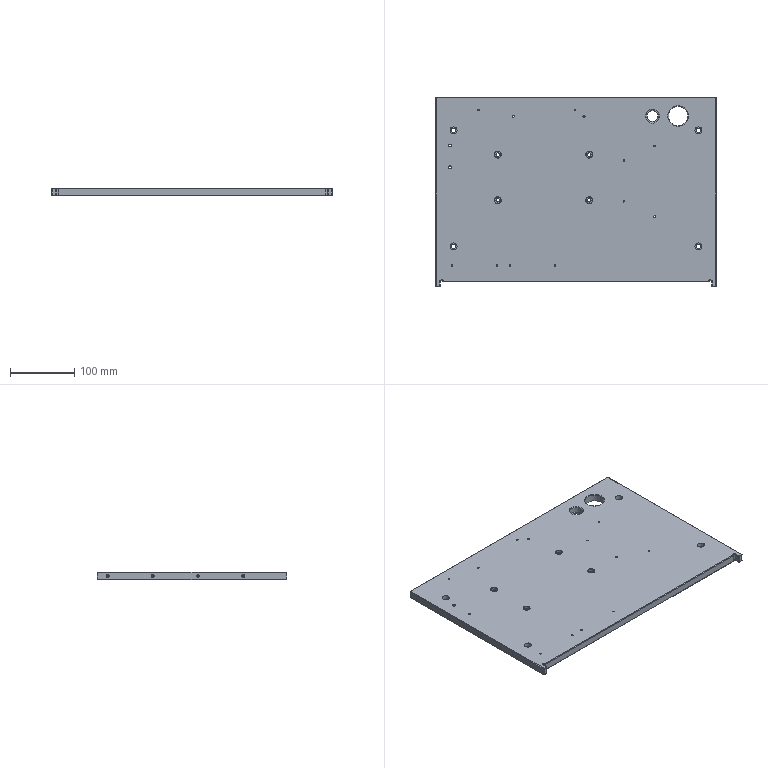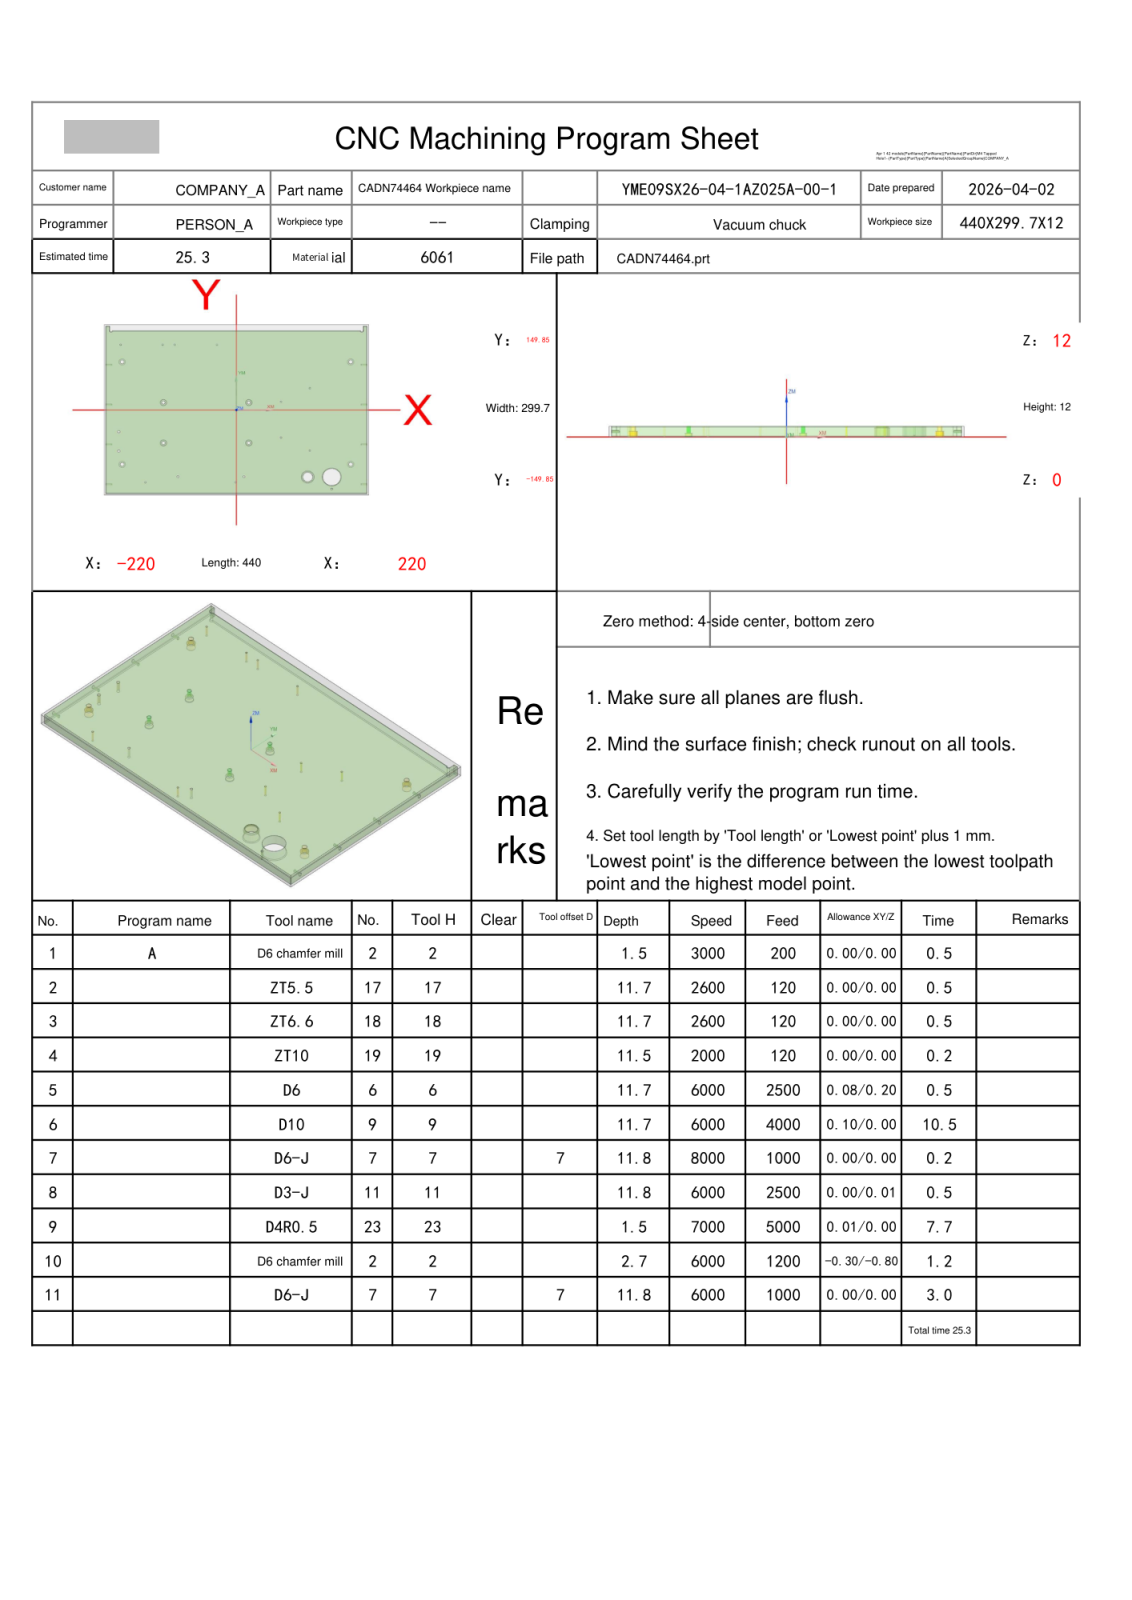NC program | NX | posted by the shop | part box 435 x 294.7 x 12 mm
Lines 3076 to 4772 of 24066:
N9 T23 M06
(D4R0.5  D=4. R=0.5 H=23 ce=0.01 di=0.00)
G00 G90 G54 X218.164 Y-120.194 M03 S7000
G43 H23 Z32.
M08
Z13.5
G01 Y-146.479 Z12.122 F5000.
X218.104 Y-146.811 Z12.105
X217.979 Y-147.124 Z12.087
X217.793 Y-147.405 Z12.069
X217.555 Y-147.643 Z12.052
X217.274 Y-147.829 Z12.034
X216.961 Y-147.954 Z12.016
X216.629 Y-148.014 Z11.999
X216.5 Z11.992
X-216.5
G02 X-218.164 Y-146.35 I0.0 J1.664
G01 Y146.35
G02 X-216.5 Y148.014 I1.664 J0.0
G01 X-211.5
G02 X-209.836 Y146.35 I0.0 J-1.664
G01 Y139.35
G03 X-208.5 Y138.014 I1.336 J0.0
X-207.23 Y138.937 I0.0 J1.336
G02 X-205.744 Y140.014 I1.486 J-.486
G01 X-205.742
X205.742
X205.744
G02 X207.23 Y138.937 I0.0 J-1.563
G03 X208.5 Y138.014 I1.27 J.413
X209.836 Y139.35 I0.0 J1.336
G01 Y146.35
G02 X211.5 Y148.014 I1.664 J0.0
G01 X216.5
G02 X218.164 Y146.35 I0.0 J-1.664
G01 Y-146.35
G02 X216.5 Y-148.014 I-1.664 J0.0
G01 X214.495
X212.491
X210.486 Y-148.015
X208.481 Y-148.014
X206.477 Y-148.015
X204.472 Y-148.014
X202.468 Y-148.015
X200.463
X198.458 Y-148.016
X196.454 Y-148.015
X194.449 Y-148.016
X192.444 Y-148.015
X190.44 Y-148.016
X188.435
X186.431
X184.426
X182.421 Y-148.017
X180.417 Y-148.016
X178.412 Y-148.017
X176.407
X174.403
X172.398
X170.394 Y-148.018
X168.389 Y-148.017
X166.384 Y-148.018
X164.38
X162.375
X160.37
X158.366 Y-148.019
X156.361 Y-148.018
X154.356 Y-148.019
X152.352
X150.347
X148.343 Z11.991
X146.338 Y-148.02
X144.333 Y-148.019
X142.329 Y-148.02
X140.324
X138.319
X136.315
X134.31 Y-148.021
X132.306 Y-148.02
X130.301 Y-148.021
X128.296
X126.292
X124.287
X122.282 Y-148.022
X120.278 Y-148.021
X118.273 Y-148.022
X116.269
X114.264
X112.259
X110.255 Y-148.023
X108.25 Y-148.022
X106.245 Y-148.023
X104.241
X102.236
X100.231
X98.227
X96.222
X94.218 Y-148.024
X92.213
X90.208
X88.204
X86.199
X84.194
X82.19 Y-148.025
X80.185
X78.181
X76.176
X74.171
X72.167
X70.162 Y-148.026
X68.157
X66.153
X64.148
X62.144
X60.139
X58.134 Y-148.027
X56.13
X54.125
X52.12
X50.116
X48.111
X46.106 Y-148.028
X44.102
X42.097
X40.093
X38.088
X36.083
X34.079
X32.074
X30.069 Y-148.029 Z11.99
X28.065
X26.06
X24.056
X22.051
X20.046
X18.042 Y-148.03
X16.037
X14.032
X12.028
X10.023
X8.019
X6.014
X4.009
X2.005 Y-148.031
X0.0
X-2.005
X-4.009
X-6.014
X-8.019
X-10.023 Y-148.032
X-12.028 Y-148.031
X-14.032 Y-148.032
X-16.037
X-18.042
X-20.046
X-22.051 Y-148.033
X-24.056 Y-148.032
X-26.06 Y-148.033
X-28.065
X-30.069
X-32.074
X-34.079
X-36.083
X-38.088 Y-148.034
X-40.093 Y-148.033
X-42.097 Y-148.034
X-44.102
X-46.106
X-48.111
X-50.116 Y-148.035
X-52.12 Y-148.034
X-54.125 Y-148.035
X-56.13 Y-148.034
X-58.134 Y-148.035
X-60.139
X-62.144
X-64.148
X-66.153 Y-148.036
X-68.157 Y-148.035
X-70.162 Y-148.036
X-72.167
X-74.171
X-76.176
X-78.181 Y-148.037
X-80.185 Y-148.036
X-82.19 Y-148.037
X-84.194 Y-148.036
X-86.199 Y-148.037
X-88.204 Z11.989
X-90.208
X-92.213
X-94.218 Y-148.038
X-96.222 Y-148.037
X-98.227 Y-148.038
X-100.231 Y-148.037
X-102.236 Y-148.038
X-104.241
X-106.245 Y-148.039
X-108.25 Y-148.038
X-110.255 Y-148.039
X-112.259 Y-148.038
X-114.264 Y-148.039
X-116.269
X-118.273
X-120.278
X-122.282 Y-148.04
X-124.287 Y-148.039
X-126.292 Y-148.04
X-128.296 Y-148.039
X-130.301 Y-148.04
X-132.306
X-134.31
X-136.315
X-138.319 Y-148.041
X-140.324 Y-148.04
X-142.329 Y-148.041
X-144.333
X-146.338
X-148.343
X-150.347 Y-148.042
X-152.352 Y-148.041
X-154.356 Y-148.042
X-156.361 Y-148.041
X-158.366 Y-148.042
X-160.37
X-162.375
X-164.38
X-166.384 Y-148.043
X-168.389 Y-148.042
X-170.394 Y-148.043
X-172.398 Y-148.042
X-174.403 Y-148.043
X-176.407
X-178.412 Y-148.044
X-180.417 Y-148.043
X-182.421 Y-148.044
X-184.426 Y-148.043
X-186.431 Y-148.044
X-188.435
X-190.44
X-192.444
X-194.449 Y-148.045
X-196.454 Y-148.044
X-198.458 Y-148.045
X-200.463 Y-148.044
X-202.468 Y-148.045
X-204.472
X-206.477 Z11.988
X-208.481
X-210.486 Y-148.046
X-212.491 Y-148.045
X-214.495 Y-148.046
X-216.5 Y-148.045
X-216.621 Y-148.042
X-216.741 Y-148.028
X-216.86 Y-148.007
X-216.978 Y-147.977
X-217.093 Y-147.939
X-217.204 Y-147.892
X-217.313 Y-147.838
X-217.417 Y-147.776
X-217.516 Y-147.708
X-217.61 Y-147.631
X-217.699 Y-147.549
X-217.781 Y-147.46
X-217.858 Y-147.366
X-217.926 Y-147.267
X-217.989 Y-147.163
X-218.042 Y-147.054
X-218.089 Y-146.943
X-218.127 Y-146.828
X-218.157 Y-146.711
X-218.178 Y-146.591
X-218.192 Y-146.471
X-218.196 Y-146.35
Y-144.345
Y-142.34
X-218.197 Y-140.336
X-218.196 Y-138.331
X-218.197 Y-136.326
X-218.196 Y-134.321
X-218.197 Y-132.316
Y-130.312
X-218.198 Y-128.307
X-218.197 Y-126.302
X-218.198 Y-124.297
X-218.197 Y-122.292
X-218.198 Y-120.288
Y-118.283
Y-116.278
Y-114.273
X-218.199 Y-112.268
X-218.198 Y-110.264
X-218.199 Y-108.259
X-218.198 Y-106.254
X-218.199 Y-104.249
Y-102.245
Y-100.24
Y-98.235
X-218.2 Y-96.23
X-218.199 Y-94.225
X-218.2 Y-92.221
X-218.199 Y-90.216
X-218.2 Y-88.211
Y-86.206
Y-84.201
Y-82.197
X-218.201 Y-80.192
X-218.2 Y-78.187
X-218.201 Y-76.182
Y-74.177
Y-72.173
Y-70.168
X-218.202 Y-68.163
X-218.201 Y-66.158
X-218.202 Y-64.153
X-218.201 Y-62.149
X-218.202 Y-60.144
Y-58.139
Y-56.134
Y-54.129
X-218.203 Y-52.125
X-218.202 Y-50.12
X-218.203 Y-48.115
X-218.202 Y-46.11
X-218.203 Y-44.105
Y-42.101 Z11.987
Y-40.096
Y-38.091
X-218.204 Y-36.086
X-218.203 Y-34.082
X-218.204 Y-32.077
Y-30.072
Y-28.067
Y-26.062
Y-24.058
Y-22.053
X-218.205 Y-20.048
X-218.204 Y-18.043
X-218.205 Y-16.038
Y-14.034
Y-12.029
Y-10.024
Y-8.019
Y-6.014
X-218.206 Y-4.01
Y-2.005
Y0.0
Y2.005
Y4.01
Y6.014
Y8.019
Y10.024
X-218.207 Y12.029
Y14.034
Y16.038
Y18.043
Y20.048
Y22.053
X-218.208 Y24.058
X-218.207 Y26.062
X-218.208 Y28.067
Y30.072
Y32.077
Y34.082
Y36.086
Y38.091
X-218.209 Y40.096
Y42.101
Y44.105
Y46.11
Y48.115
Y50.12
Y52.125
Y54.129
X-218.21 Y56.134
Y58.139
Y60.144
Y62.149
Y64.153
Y66.158
Y68.163
Y70.168
X-218.211 Y72.173
Y74.177
Y76.182 Z11.986
Y78.187
Y80.192
Y82.197
Y84.201
Y86.206
X-218.212 Y88.211
Y90.216
Y92.221
Y94.225
Y96.23
Y98.235
Y100.24
Y102.245
X-218.213 Y104.249
Y106.254
Y108.259
Y110.264
Y112.268
Y114.273
Y116.278
Y118.283
X-218.214 Y120.288
X-218.213 Y122.292
X-218.214 Y124.297
Y126.302
Y128.307
Y130.312
Y132.316
Y134.321
X-218.215 Y136.326
X-218.214 Y138.331
X-218.215 Y140.336
Y142.34
Y144.345
Y146.35
X-218.211 Y146.472
X-218.197 Y146.594
X-218.176 Y146.715
X-218.145 Y146.833
X-218.107 Y146.949
X-218.06 Y147.062
X-218.005 Y147.172
X-217.943 Y147.277
X-217.873 Y147.378
X-217.796 Y147.473
X-217.713 Y147.563
X-217.623 Y147.646
X-217.528 Y147.723
X-217.427 Y147.793
X-217.322 Y147.855
X-217.212 Y147.91
X-217.099 Y147.957
X-216.983 Y147.996
X-216.865 Y148.026
X-216.744 Y148.048
X-216.622 Y148.061
X-216.5 Y148.065
X-215.25
X-214.
X-212.75
X-211.5
X-211.378 Y148.061
X-211.256 Y148.048
X-211.135 Y148.026
X-211.017 Y147.996
X-210.901 Y147.957
X-210.787 Y147.91
X-210.678 Y147.856
X-210.573 Y147.793
X-210.472 Y147.723
X-210.377 Y147.646
X-210.287 Y147.563
X-210.204 Y147.473
X-210.127 Y147.378
X-210.057 Y147.277
X-209.994 Y147.172
X-209.94 Y147.063
X-209.893 Y146.949
X-209.854 Y146.833
X-209.824 Y146.715
X-209.802 Y146.594
X-209.789 Y146.472
X-209.785 Y146.35
Y144.6
X-209.784 Y142.85
X-209.785 Y141.1
X-209.784 Y139.35
X-209.78 Y139.251
X-209.769 Y139.152
X-209.75 Y139.055
X-209.723 Y138.959
X-209.689 Y138.866
X-209.648 Y138.775
X-209.6 Y138.688
X-209.546 Y138.605
X-209.485 Y138.527
X-209.419 Y138.453
X-209.346 Y138.385
X-209.269 Y138.322
X-209.188 Y138.266
X-209.102 Y138.216
X-209.01 Y138.172
X-208.915 Y138.135
X-208.818 Y138.106
X-208.718 Y138.085
X-208.617 Y138.071
X-208.516 Y138.066
X-208.414 Y138.069
X-208.313 Y138.08
X-208.213 Y138.099
X-208.115 Y138.125
X-208.019 Y138.16
X-207.926 Y138.201
X-207.837 Y138.251
X-207.752 Y138.307
X-207.672 Y138.369
X-207.597 Y138.438
X-207.527 Y138.512
X-207.464 Y138.592
X-207.407 Y138.676
X-207.357 Y138.765
X-207.315 Y138.857
X-207.276 Y138.963
X-207.273 Y138.973
X-207.233 Y139.082
X-207.186 Y139.187
X-207.157 Y139.244
X-207.125 Y139.298
X-207.092 Y139.353
X-207.055 Y139.406
X-207.018 Y139.457
X-206.978 Y139.506
X-206.935 Y139.555
X-206.891 Y139.601
X-206.845 Y139.646
X-206.798 Y139.688
X-206.748 Y139.729
X-206.697 Y139.767
X-206.645 Y139.804
X-206.59 Y139.838
X-206.535 Y139.87
X-206.479 Y139.9
X-206.421 Y139.927
X-206.362 Y139.952
X-206.303 Y139.975
X-206.242 Y139.995
X-206.181 Y140.013
X-206.118 Y140.028
X-206.056 Y140.041
X-205.994 Y140.051
X-205.891 Y140.062
X-205.788 Y140.066
X-205.765 Y140.067
X-205.742 Y140.066
X-203.744 Y140.065
X-201.747 Y140.066
X-199.749
X-197.752 Y140.067
X-195.754 Y140.066
X-193.757 Y140.067
X-191.759 Y140.066
X-189.762 Y140.067
X-187.765 Y140.066
X-185.767 Y140.067
X-183.77
X-181.772 Y140.068
X-179.775 Y140.067 Z11.985
X-177.777 Y140.068
X-175.78 Y140.067
X-173.782 Y140.068
X-171.785 Y140.067
X-169.787 Y140.068
X-167.79
X-165.792 Y140.069
X-163.795 Y140.068
X-161.797 Y140.069
X-159.8 Y140.068
X-157.802 Y140.069
X-155.805 Y140.068
X-153.807 Y140.069
X-151.81
X-149.812
X-147.815
X-145.817 Y140.07
X-143.82 Y140.069
X-141.822 Y140.07
X-139.825 Y140.069
X-137.827 Y140.07
X-135.83 Y140.069
X-133.832 Y140.07
X-131.835
X-129.837 Y140.071
X-127.84 Y140.07
X-125.842 Y140.071
X-123.845 Y140.07
X-121.847 Y140.071
X-119.85 Y140.07
X-117.852 Y140.071
X-115.855
X-113.857 Y140.072
X-111.86 Y140.071
X-109.862 Y140.072
X-107.865 Y140.071
X-105.867 Y140.072
X-103.87 Y140.071
X-101.872 Y140.072
X-99.875
X-97.877
X-95.88
X-93.882 Y140.073
X-91.885 Y140.072
X-89.887 Y140.073
X-87.89 Y140.072
X-85.892 Y140.073
X-83.895
X-81.897
X-79.9
X-77.902 Y140.074
X-75.905 Y140.073
X-73.907 Y140.074
X-71.91 Y140.073
X-69.912 Y140.074
X-67.915
X-65.917
X-63.92
X-61.922 Y140.075 Z11.984
X-59.925 Y140.074
X-57.927 Y140.075
X-55.93 Y140.074
X-53.932 Y140.075
X-51.935
X-49.937
X-47.94
X-45.942
X-43.945
X-41.947 Y140.076
X-39.95 Y140.075
X-37.952 Y140.076
X-35.955
X-33.957
X-31.96
X-29.962
X-27.965
X-25.967 Y140.077
X-23.97 Y140.076
X-21.972 Y140.077
X-19.975
X-17.977
X-15.98
X-13.982
X-11.985
X-9.987 Y140.078
X-7.99 Y140.077
X-5.992 Y140.078
X-3.995
X-1.997
X0.0
X1.997
X3.995
X5.992
X7.99
X9.987 Y140.079
X11.985 Y140.078
X13.982 Y140.079
X15.98
X17.977
X19.975
X21.972
X23.97
X25.967 Y140.08
X27.965 Y140.079
X29.962 Y140.08
X31.96
X33.957
X35.955
X37.952
X39.95
X41.947 Y140.081
X43.945 Y140.08
X45.942 Y140.081
X47.94
X49.937
X51.935
X53.932
X55.93 Z11.983
X57.927
X59.925
X61.922 Y140.082
X63.92
X65.917
X67.915
X69.912
X71.91
X73.907
X75.905
X77.902 Y140.083
X79.9
X81.897
X83.895
X85.892
X87.89
X89.887
X91.885
X93.882 Y140.084
X95.88
X97.877
X99.875
X101.872
X103.87
X105.867
X107.865
X109.862
X111.86 Y140.085
X113.857
X115.855
X117.852
X119.85
X121.847
X123.845
X125.842
X127.84 Y140.086
X129.837
X131.835
X133.832
X135.83
X137.827
X139.825
X141.822
X143.82 Y140.087
X145.817
X147.815
X149.812
X151.81
X153.807
X155.805
X157.802
X159.8 Y140.088
X161.797 Y140.087
X163.795 Y140.088
X165.792
X167.79
X169.787
X171.785
X173.782 Z11.982
X175.78
X177.777
X179.775 Y140.089
X181.772
X183.77
X185.767
X187.765
X189.762
X191.759
X193.757
X195.754 Y140.09
X197.752
X199.749
X201.747
X203.744
X205.742
X205.765
X205.788 Y140.089
X205.893 Y140.086
X205.997 Y140.076
X206.061 Y140.066
X206.124 Y140.053
X206.187 Y140.038
X206.25 Y140.02
X206.312 Y140.
X206.372 Y139.977
X206.432 Y139.952
X206.491 Y139.924
X206.549 Y139.894
X206.605 Y139.862
X206.66 Y139.827
X206.714 Y139.79
X206.765 Y139.751
X206.816 Y139.709
X206.864 Y139.666
X206.911 Y139.621
X206.956 Y139.573
X206.998 Y139.524
X207.039 Y139.474
X207.078 Y139.421
X207.114 Y139.368
X207.148 Y139.312
X207.18 Y139.256
X207.209 Y139.198
X207.256 Y139.091
X207.295 Y138.98
X207.302 Y138.96
X207.335 Y138.869
X207.376 Y138.781
X207.423 Y138.697
X207.476 Y138.616
X207.536 Y138.54
X207.601 Y138.468
X207.671 Y138.401
X207.746 Y138.341
X207.826 Y138.286
X207.91 Y138.237
X208.007 Y138.191
X208.108 Y138.153
X208.212 Y138.123
X208.318 Y138.103
X208.426 Y138.092
X208.534 Y138.091
X208.642 Y138.098
X208.748 Y138.115
X208.853 Y138.141
X208.956 Y138.175
X209.054 Y138.219
X209.149 Y138.27
X209.239 Y138.33
X209.324 Y138.397
X209.403 Y138.471
X209.475 Y138.552
X209.539 Y138.638
X209.597 Y138.73
X209.646 Y138.826
X209.686 Y138.926
X209.718 Y139.029
X209.741 Y139.135
X209.755 Y139.242
X209.76 Y139.35
Y141.1
Y142.85
Y144.6
X209.759 Y146.35
X209.764 Y146.474
X209.777 Y146.598
X209.799 Y146.72
X209.83 Y146.84
X209.869 Y146.958
X209.917 Y147.073
X209.972 Y147.184
X210.036 Y147.291
X210.106 Y147.393
X210.184 Y147.49
X210.269 Y147.581
X210.36 Y147.666
X210.457 Y147.744
X210.559 Y147.814
X210.666 Y147.878
X210.777 Y147.934
X210.892 Y147.981
X211.01 Y148.02
X211.13 Y148.051
X211.252 Y148.073
X211.376 Y148.086
X211.5 Y148.091
X212.75
X214.
X215.25
X216.5
X216.624 Y148.087
X216.748 Y148.073
X216.87 Y148.051
X216.991 Y148.021
X217.108 Y147.981
X217.223 Y147.934
X217.334 Y147.878
X217.441 Y147.815
X217.543 Y147.744
X217.64 Y147.666
X217.731 Y147.581
X217.816 Y147.49
X217.894 Y147.393
X217.965 Y147.291
X218.028 Y147.184
X218.084 Y147.073
X218.131 Y146.958
X218.171 Y146.841
X218.201 Y146.72
X218.224 Y146.598
X218.237 Y146.474
X218.241 Y146.35
X218.242 Y144.345
Y142.34
Y140.336
Y138.331
Y136.326
Y134.321
Y132.316
Y130.312
Y128.307
Y126.302
X218.243 Y124.297
Y122.292
Y120.288
Y118.283
Y116.278
Y114.273
Y112.268
Y110.264
X218.244 Y108.259
Y106.254
Y104.249
Y102.245
Y100.24
Y98.235
Y96.23
Y94.225
Y92.221
Y90.216
X218.245 Y88.211
Y86.206
Y84.201
Y82.197 Z11.981
Y80.192
Y78.187
Y76.182
Y74.177
Y72.173
Y70.168
X218.246 Y68.163
Y66.158
Y64.153
Y62.149
Y60.144
Y58.139
Y56.134
Y54.129
X218.247 Y52.125
X218.246 Y50.12
X218.247 Y48.115
Y46.11
Y44.105
Y42.101
Y40.096
Y38.091
Y36.086
Y34.082
X218.248 Y32.077
X218.247 Y30.072
X218.248 Y28.067
Y26.062
Y24.058
Y22.053
Y20.048
Y18.043
Y16.038
Y14.034
X218.249 Y12.029
X218.248 Y10.024
X218.249 Y8.019
Y6.014
Y4.01
Y2.005
Y0.0
Y-2.005
Y-4.01
Y-6.014
X218.25 Y-8.019
X218.249 Y-10.024
X218.25 Y-12.029
Y-14.034
Y-16.038
Y-18.043
Y-20.048
Y-22.053
X218.251 Y-24.058
X218.25 Y-26.062
X218.251 Y-28.067
X218.25 Y-30.072
X218.251 Y-32.077
Y-34.082
Y-36.086 Z11.98
Y-38.091
Y-40.096
Y-42.101
X218.252 Y-44.105
X218.251 Y-46.11
X218.252 Y-48.115
X218.251 Y-50.12
X218.252 Y-52.125
Y-54.129
Y-56.134
Y-58.139
Y-60.144
Y-62.149
X218.253 Y-64.153
X218.252 Y-66.158
X218.253 Y-68.163
X218.252 Y-70.168
X218.253 Y-72.173
Y-74.177
Y-76.182
Y-78.187
Y-80.192
Y-82.197
X218.254 Y-84.201
X218.253 Y-86.206
X218.254 Y-88.211
X218.253 Y-90.216
X218.254 Y-92.221
Y-94.225
Y-96.23
Y-98.235
Y-100.24
Y-102.245
X218.255 Y-104.249
X218.254 Y-106.254
X218.255 Y-108.259
X218.254 Y-110.264
X218.255 Y-112.268
Y-114.273
Y-116.278
Y-118.283
Y-120.288
Y-122.292
X218.256 Y-124.297
X218.255 Y-126.302
X218.256 Y-128.307
X218.255 Y-130.312
X218.256 Y-132.316
Y-134.321
Y-136.326
Y-138.331
Y-140.336
Y-142.34
X218.257 Y-144.345
X218.256 Y-146.35
X218.252 Y-146.475
X218.238 Y-146.6
X218.216 Y-146.723
X218.185 Y-146.845
X218.146 Y-146.964
X218.098 Y-147.08
X218.042 Y-147.192
X217.978 Y-147.3
X217.906 Y-147.403
X217.827 Y-147.5
X217.742 Y-147.592
X217.65 Y-147.677
X217.553 Y-147.756
X217.45 Y-147.828
X217.342 Y-147.892
X217.23 Y-147.948
X217.114 Y-147.996
X216.995 Y-148.035
X216.873 Y-148.067
X216.75 Y-148.089
X216.625 Y-148.102
X216.5 Y-148.107
X214.495
X212.491 Z11.979
X210.486
X208.481
X206.477 Y-148.108
X204.472 Y-148.107
X202.468 Y-148.108
X200.463
X198.458
X196.454
X194.449
X192.444
X190.44 Y-148.109
X188.435 Y-148.108
X186.431 Y-148.109
X184.426
X182.421
X180.417
X178.412 Y-148.11
X176.407 Y-148.109
X174.403 Y-148.11
X172.398
X170.394
X168.389
X166.384
X164.38
X162.375 Y-148.111
X160.37 Y-148.11
X158.366 Y-148.111
X156.361
X154.356
X152.352
X150.347 Y-148.112
X148.343 Y-148.111
X146.338 Y-148.112
X144.333
X142.329
X140.324
X138.319
X136.315
X134.31 Y-148.113
X132.306
X130.301
X128.296 Z11.978
X126.292
X124.287
X122.282 Y-148.114
X120.278 Y-148.113
X118.273 Y-148.114
X116.269
X114.264
X112.259
X110.255
X108.25
X106.245 Y-148.115
X104.241
X102.236
X100.231
X98.227
X96.222
X94.218
X92.213
X90.208 Y-148.116
X88.204
X86.199
X84.194
X82.19
X80.185
X78.181 Y-148.117
X76.176
X74.171
X72.167
X70.162
X68.157
X66.153
X64.148
X62.144 Y-148.118
X60.139
X58.134
X56.13
X54.125
X52.12
X50.116
X48.111 Y-148.119
X46.106
X44.102 Z11.977
X42.097
X40.093
X38.088
X36.083
X34.079 Y-148.12
X32.074
X30.069
X28.065
X26.06
X24.056
X22.051
X20.046
X18.042 Y-148.121
X16.037
X14.032
X12.028
X10.023
X8.019
X6.014
X4.009
X2.005 Y-148.122
X0.0
X-2.005
X-4.009
X-6.014
X-8.019
X-10.023
X-12.028
X-14.032 Y-148.123
X-16.037
X-18.042
X-20.046
X-22.051
X-24.056
X-26.06 Y-148.124
X-28.065 Y-148.123
X-30.069 Y-148.124
X-32.074
X-34.079
X-36.083
X-38.088
X-40.093
X-42.097 Y-148.125 Z11.976
X-44.102 Y-148.124
X-46.106 Y-148.125
X-48.111
X-50.116
X-52.12
X-54.125
X-56.13
X-58.134 Y-148.126
X-60.139 Y-148.125
X-62.144 Y-148.126
X-64.148
X-66.153
X-68.157
X-70.162
X-72.167
X-74.171 Y-148.127
X-76.176 Y-148.126
X-78.181 Y-148.127
X-80.185
X-82.19
X-84.194
X-86.199
X-88.204
X-90.208 Y-148.128
X-92.213 Y-148.127
X-94.218 Y-148.128
X-96.222
X-98.227
X-100.231
X-102.236 Y-148.129
X-104.241 Y-148.128
X-106.245 Y-148.129
X-108.25 Y-148.128
X-110.255 Y-148.129
X-112.259
X-114.264
X-116.269
X-118.273 Y-148.13
X-120.278 Y-148.129
X-122.282 Y-148.13
X-124.287 Y-148.129
X-126.292 Y-148.13 Z11.975
X-128.296
X-130.301
X-132.306
X-134.31 Y-148.131
X-136.315 Y-148.13
X-138.319 Y-148.131
X-140.324
X-142.329
X-144.333
X-146.338
X-148.343
X-150.347 Y-148.132
X-152.352 Y-148.131
X-154.356 Y-148.132
X-156.361
X-158.366
X-160.37
X-162.375
X-164.38
X-166.384 Y-148.133
X-168.389 Y-148.132
X-170.394 Y-148.133
X-172.398
X-174.403
X-176.407
X-178.412
X-180.417
X-182.421 Y-148.134
X-184.426 Y-148.133
X-186.431 Y-148.134
X-188.435
X-190.44
X-192.444
X-194.449
X-196.454
X-198.458 Y-148.135
X-200.463 Y-148.134
X-202.468 Y-148.135
X-204.472
X-206.477
X-208.481
X-210.486 Z11.974
X-212.491
X-214.495 Y-148.136
X-216.5 Y-148.135
X-216.627 Y-148.131
X-216.754 Y-148.117
X-216.88 Y-148.095
X-217.003 Y-148.063
X-217.124 Y-148.023
X-217.242 Y-147.974
X-217.356 Y-147.917
X-217.465 Y-147.852
X-217.57 Y-147.779
X-217.669 Y-147.699
X-217.763 Y-147.613
X-217.849 Y-147.519
X-217.93 Y-147.42
X-218.002 Y-147.315
X-218.067 Y-147.206
X-218.124 Y-147.092
X-218.173 Y-146.974
X-218.213 Y-146.853
X-218.245 Y-146.73
X-218.267 Y-146.604
X-218.281 Y-146.477
X-218.286 Y-146.35
Y-144.345
Y-142.34
Y-140.336
Y-138.331
X-218.287 Y-136.326
X-218.286 Y-134.321
X-218.287 Y-132.316
Y-130.312
Y-128.307
Y-126.302
Y-124.297
Y-122.292
X-218.288 Y-120.288
X-218.287 Y-118.283
X-218.288 Y-116.278
Y-114.273
Y-112.268
Y-110.264
Y-108.259
Y-106.254
X-218.289 Y-104.249
X-218.288 Y-102.245
X-218.289 Y-100.24
Y-98.235
Y-96.23
Y-94.225
Y-92.221
Y-90.216
X-218.29 Y-88.211
X-218.289 Y-86.206
X-218.29 Y-84.201
Y-82.197
Y-80.192
Y-78.187
Y-76.182
Y-74.177
X-218.291 Y-72.173
X-218.29 Y-70.168 Z11.973
X-218.291 Y-68.163
Y-66.158
Y-64.153
Y-62.149
Y-60.144
Y-58.139
X-218.292 Y-56.134
X-218.291 Y-54.129
X-218.292 Y-52.125
Y-50.12
Y-48.115
Y-46.11
Y-44.105
Y-42.101
X-218.293 Y-40.096
X-218.292 Y-38.091
X-218.293 Y-36.086
Y-34.082
Y-32.077
Y-30.072
Y-28.067
Y-26.062
X-218.294 Y-24.058
X-218.293 Y-22.053
X-218.294 Y-20.048
Y-18.043
Y-16.038
Y-14.034
Y-12.029
Y-10.024
X-218.295 Y-8.019
X-218.294 Y-6.014
X-218.295 Y-4.01
Y-2.005
Y0.0
Y2.005
Y4.01
Y6.014
X-218.296 Y8.019
X-218.295 Y10.024
X-218.296 Y12.029
Y14.034 Z11.972
Y16.038
Y18.043
Y20.048
Y22.053
X-218.297 Y24.058
X-218.296 Y26.062
X-218.297 Y28.067
Y30.072
Y32.077
Y34.082
Y36.086
Y38.091
X-218.298 Y40.096
X-218.297 Y42.101
X-218.298 Y44.105
Y46.11
Y48.115
Y50.12
Y52.125
Y54.129
Y56.134
Y58.139
X-218.299 Y60.144
Y62.149
Y64.153
Y66.158
Y68.163
Y70.168
Y72.173
X-218.3 Y74.177
Y76.182
Y78.187
Y80.192
Y82.197
Y84.201
Y86.206
Y88.211
X-218.301 Y90.216
Y92.221
Y94.225
Y96.23
Y98.235 Z11.971
Y100.24
Y102.245
Y104.249
Y106.254
X-218.302 Y108.259
Y110.264
Y112.268
Y114.273
Y116.278
Y118.283
Y120.288
Y122.292
X-218.303 Y124.297
Y126.302
Y128.307
Y130.312
Y132.316
Y134.321
Y136.326
Y138.331
X-218.304 Y140.336
Y142.34
Y144.345
Y146.35
X-218.299 Y146.479
X-218.285 Y146.607
X-218.262 Y146.733
X-218.231 Y146.858
X-218.19 Y146.98
X-218.141 Y147.099
X-218.083 Y147.214
X-218.017 Y147.325
X-217.944 Y147.431
X-217.863 Y147.531
X-217.775 Y147.625
X-217.681 Y147.713
X-217.581 Y147.794
X-217.475 Y147.867
X-217.364 Y147.933
X-217.249 Y147.991
X-217.13 Y148.04
X-217.008 Y148.081
X-216.883 Y148.113
X-216.757 Y148.136
X-216.629 Y148.149
X-216.5 Y148.154
X-215.25
X-214.
X-212.75
X-211.5
X-211.371 Y148.15
X-211.243 Y148.136
X-211.117 Y148.113
X-210.992 Y148.081
X-210.87 Y148.04
X-210.75 Y147.991
X-210.635 Y147.933
X-210.525 Y147.868
X-210.419 Y147.794
X-210.318 Y147.714
X-210.224 Y147.626
X-210.136 Y147.532
X-210.056 Y147.431
X-209.982 Y147.325
X-209.916 Y147.215
X-209.859 Y147.1
X-209.81 Y146.981
X-209.769 Y146.858
X-209.737 Y146.734
X-209.714 Y146.607
X-209.7 Y146.479
X-209.696 Y146.35
X-209.695 Y144.6
Y142.85
Y141.1
Y139.35
X-209.69 Y139.243
X-209.676 Y139.138
X-209.653 Y139.033
X-209.62 Y138.932
X-209.578 Y138.834
X-209.527 Y138.739
X-209.469 Y138.65
X-209.403 Y138.566
X-209.329 Y138.489
X-209.249 Y138.418
X-209.208 Y138.387
X-209.165 Y138.357
X-209.119 Y138.328
X-209.071 Y138.3
X-208.975 Y138.253
X-208.876 Y138.215
X-208.774 Y138.187
X-208.67 Y138.167
X-208.565 Y138.157
X-208.459 Y138.156
X-208.353 Y138.164
X-208.249 Y138.181
X-208.147 Y138.208
X-208.047 Y138.244
X-207.951 Y138.288
X-207.86 Y138.341
X-207.773 Y138.401
X-207.692 Y138.469
X-207.617 Y138.544
X-207.55 Y138.626
X-207.489 Y138.712
X-207.437 Y138.804
X-207.393 Y138.9
X-207.352 Y139.017
X-207.318 Y139.118
X-207.277 Y139.216
X-207.225 Y139.32
X-207.166 Y139.42
X-207.099 Y139.516
X-207.026 Y139.607
X-206.946 Y139.692
X-206.86 Y139.771
X-206.769 Y139.843
X-206.672 Y139.909
X-206.571 Y139.968
X-206.466 Y140.018
X-206.358 Y140.062
X-206.247 Y140.097
X-206.134 Y140.124
X-206.019 Y140.142
X-205.925 Y140.152
X-205.831 Y140.155
X-205.81
X-205.789
X-203.791 Y140.154
X-201.793 Y140.155
X-199.795
X-197.797 Y140.156
X-195.799 Y140.155
X-193.801 Y140.156
X-191.803 Y140.155 Z11.97
X-189.805 Y140.156
X-187.807 Y140.155
X-185.809 Y140.156
X-183.811
X-181.813
X-179.815
X-177.817 Y140.157
X-175.819 Y140.156
X-173.822 Y140.157
X-171.824 Y140.156
X-169.826 Y140.157
X-167.828
X-165.83
X-163.832
X-161.834 Y140.158
X-159.836 Y140.157
X-157.838 Y140.158
X-155.84 Y140.157
X-153.842 Y140.158
X-151.844 Y140.157
X-149.846 Y140.158
X-147.848
X-145.85
X-143.852
X-141.854 Y140.159
X-139.856 Y140.158
X-137.858 Y140.159
X-135.861 Y140.158
X-133.863 Y140.159
X-131.865
X-129.867
X-127.869
X-125.871 Y140.16
X-123.873 Y140.159
X-121.875 Y140.16
X-119.877 Y140.159
X-117.879 Y140.16
X-115.881
X-113.883
X-111.885
X-109.887
X-107.889 Z11.969
X-105.891 Y140.161
X-103.893 Y140.16
X-101.895 Y140.161
X-99.897 Y140.16
X-97.899 Y140.161
X-95.902
X-93.904
X-91.906
X-89.908 Y140.162
X-87.91 Y140.161
X-85.912 Y140.162
X-83.914 Y140.161
X-81.916 Y140.162
X-79.918
X-77.92
X-75.922
X-73.924
X-71.926
X-69.928 Y140.163
X-67.93 Y140.162
X-65.932 Y140.163
X-63.934
X-61.936
X-59.938
X-57.941
X-55.943
X-53.945 Y140.164
X-51.947 Y140.163
X-49.949 Y140.164
X-47.951 Y140.163
X-45.953 Y140.164
X-43.955
X-41.957
X-39.959
X-37.961 Y140.165
X-35.963 Y140.164
X-33.965 Y140.165
X-31.967 Y140.164
X-29.969 Y140.165
X-27.971
X-25.973
X-23.975
X-21.977 Z11.968
X-19.979
X-17.982 Y140.166
X-15.984 Y140.165
X-13.986 Y140.166
X-11.988
X-9.99
X-7.992
X-5.994
X-3.996
X-1.998 Y140.167
X0.0 Y140.166
X1.998 Y140.167
X3.996 Y140.166
X5.994 Y140.167
X7.992
X9.99
X11.988
X13.986
X15.984
X17.982 Y140.168
X19.979 Y140.167
X21.977 Y140.168
X23.975
X25.973
X27.971
X29.969
X31.967
X33.965 Y140.169
X35.963 Y140.168
X37.961 Y140.169
X39.959
X41.957
X43.955
X45.953
X47.951
X49.949
X51.947
X53.945 Y140.17
X55.943 Y140.169
X57.941 Y140.17
X59.938
X61.936 Z11.967
X63.934
X65.932
X67.93
X69.928 Y140.171
X71.926 Y140.17
X73.924 Y140.171
X75.922
X77.92
X79.918
X81.916
X83.914
X85.912
X87.91
X89.908 Y140.172
X91.906
X93.904
X95.902
X97.899
X99.897
X101.895
X103.893
X105.891 Y140.173
X107.889 Y140.172
X109.887 Y140.173
X111.885
X113.883
X115.881
X117.879
X119.877
X121.875 Y140.174
X123.873 Y140.173
X125.871 Y140.174
X127.869
X129.867
X131.865
X133.863
X135.861
X137.858
X139.856
X141.854 Y140.175
X143.852
X145.85